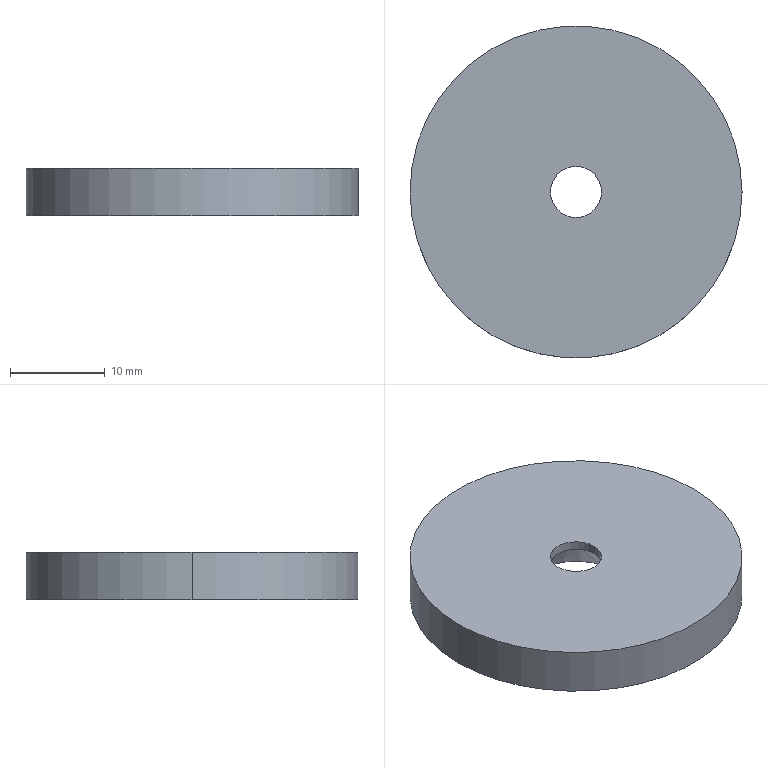Part | Creo | 1 solid | 8 faces | box 35 x 35 x 5 mm | volume 4524 mm3 | cylinder 4 | plane 2 | cone 2 | commonest cylinder face diameters 5.4 x2 35 x2
STEP:
#1=CARTESIAN_POINT('',(0.,0.,0.));
#2=DIRECTION('',(0.,0.,1.));
#3=DIRECTION('',(1.,0.,0.));
#4=AXIS2_PLACEMENT_3D('',#1,#2,#3);
#5=CARTESIAN_POINT('',(426.601,-277.627,-28.441));
#6=VERTEX_POINT('',#5);
#7=CARTESIAN_POINT('',(461.601,-277.627,-28.441));
#8=VERTEX_POINT('',#7);
#9=CARTESIAN_POINT('',(444.101,-277.627,-28.441));
#10=DIRECTION('',(0.,0.,-1.));
#11=DIRECTION('',(-1.,0.,0.));
#12=AXIS2_PLACEMENT_3D('',#9,#10,#11);
#13=CIRCLE('',#12,17.5);
#14=EDGE_CURVE('',#6,#8,#13,.T.);
#15=ORIENTED_EDGE('',*,*,#14,.F.);
#16=CARTESIAN_POINT('',(444.101,-277.627,-28.441));
#17=DIRECTION('',(0.,0.,-1.));
#18=DIRECTION('',(1.,0.,0.));
#19=AXIS2_PLACEMENT_3D('',#16,#17,#18);
#20=CIRCLE('',#19,17.5);
#21=EDGE_CURVE('',#8,#6,#20,.T.);
#22=ORIENTED_EDGE('',*,*,#21,.F.);
#23=EDGE_LOOP('',(#15,#22));
#24=FACE_OUTER_BOUND('',#23,.F.);
#25=CARTESIAN_POINT('',(450.309,-277.627,-28.441));
#26=VERTEX_POINT('',#25);
#27=CARTESIAN_POINT('',(437.892,-277.627,-28.441));
#28=VERTEX_POINT('',#27);
#29=CARTESIAN_POINT('',(444.101,-277.627,-28.441));
#30=DIRECTION('',(0.,0.,1.));
#31=DIRECTION('',(1.,0.,0.));
#32=AXIS2_PLACEMENT_3D('',#29,#30,#31);
#33=CIRCLE('',#32,6.209);
#34=EDGE_CURVE('',#26,#28,#33,.T.);
#35=ORIENTED_EDGE('',*,*,#34,.F.);
#36=CARTESIAN_POINT('',(444.101,-277.627,-28.441));
#37=DIRECTION('',(0.,0.,1.));
#38=DIRECTION('',(-1.,0.,0.));
#39=AXIS2_PLACEMENT_3D('',#36,#37,#38);
#40=CIRCLE('',#39,6.209);
#41=EDGE_CURVE('',#28,#26,#40,.T.);
#42=ORIENTED_EDGE('',*,*,#41,.F.);
#43=EDGE_LOOP('',(#35,#42));
#44=FACE_BOUND('',#43,.F.);
#45=CARTESIAN_POINT('',(444.101,-277.627,-28.441));
#46=DIRECTION('',(0.,0.,-1.));
#47=DIRECTION('',(-1.,0.,0.));
#48=AXIS2_PLACEMENT_3D('',#45,#46,#47);
#49=PLANE('',#48);
#50=ADVANCED_FACE('',(#24,#44),#49,.T.);
#51=CARTESIAN_POINT('',(446.801,-277.627,-24.405));
#52=VERTEX_POINT('',#51);
#53=CARTESIAN_POINT('',(441.401,-277.627,-24.405));
#54=VERTEX_POINT('',#53);
#55=CARTESIAN_POINT('',(444.101,-277.627,-24.405));
#56=DIRECTION('',(0.,0.,1.));
#57=DIRECTION('',(1.,0.,0.));
#58=AXIS2_PLACEMENT_3D('',#55,#56,#57);
#59=CIRCLE('',#58,2.7);
#60=EDGE_CURVE('',#52,#54,#59,.T.);
#61=ORIENTED_EDGE('',*,*,#60,.F.);
#62=CARTESIAN_POINT('',(446.801,-277.627,-24.405));
#63=DIRECTION('',(0.6561,0.,-0.7547));
#64=VECTOR('',#63,5.348);
#65=LINE('',#62,#64);
#66=EDGE_CURVE('',#52,#26,#65,.T.);
#67=ORIENTED_EDGE('',*,*,#66,.T.);
#68=ORIENTED_EDGE('',*,*,#34,.T.);
#69=CARTESIAN_POINT('',(441.401,-277.627,-24.405));
#70=DIRECTION('',(-0.6561,0.,-0.7547));
#71=VECTOR('',#70,5.348);
#72=LINE('',#69,#71);
#73=EDGE_CURVE('',#54,#28,#72,.T.);
#74=ORIENTED_EDGE('',*,*,#73,.F.);
#75=EDGE_LOOP('',(#61,#67,#68,#74));
#76=FACE_OUTER_BOUND('',#75,.F.);
#77=CARTESIAN_POINT('',(444.101,-277.627,-26.423));
#78=DIRECTION('',(0.,0.,-1.));
#79=DIRECTION('',(-1.,0.,0.));
#80=AXIS2_PLACEMENT_3D('',#77,#78,#79);
#81=CONICAL_SURFACE('',#80,4.454,41.);
#82=ADVANCED_FACE('',(#76),#81,.F.);
#83=CARTESIAN_POINT('',(441.401,-277.627,-23.441));
#84=VERTEX_POINT('',#83);
#85=CARTESIAN_POINT('',(446.801,-277.627,-23.441));
#86=VERTEX_POINT('',#85);
#87=CARTESIAN_POINT('',(444.101,-277.627,-23.441));
#88=DIRECTION('',(0.,0.,-1.));
#89=DIRECTION('',(-1.,0.,0.));
#90=AXIS2_PLACEMENT_3D('',#87,#88,#89);
#91=CIRCLE('',#90,2.7);
#92=EDGE_CURVE('',#84,#86,#91,.T.);
#93=ORIENTED_EDGE('',*,*,#92,.T.);
#94=CARTESIAN_POINT('',(446.801,-277.627,-23.441));
#95=DIRECTION('',(0.,0.,-1.));
#96=VECTOR('',#95,0.9639);
#97=LINE('',#94,#96);
#98=EDGE_CURVE('',#86,#52,#97,.T.);
#99=ORIENTED_EDGE('',*,*,#98,.T.);
#100=ORIENTED_EDGE('',*,*,#60,.T.);
#101=CARTESIAN_POINT('',(441.401,-277.627,-23.441));
#102=DIRECTION('',(0.,0.,-1.));
#103=VECTOR('',#102,0.9639);
#104=LINE('',#101,#103);
#105=EDGE_CURVE('',#84,#54,#104,.T.);
#106=ORIENTED_EDGE('',*,*,#105,.F.);
#107=EDGE_LOOP('',(#93,#99,#100,#106));
#108=FACE_OUTER_BOUND('',#107,.F.);
#109=CARTESIAN_POINT('',(444.101,-277.627,-23.441));
#110=DIRECTION('',(0.,0.,-1.));
#111=DIRECTION('',(-1.,0.,0.));
#112=AXIS2_PLACEMENT_3D('',#109,#110,#111);
#113=CYLINDRICAL_SURFACE('',#112,2.7);
#114=ADVANCED_FACE('',(#108),#113,.F.);
#115=CARTESIAN_POINT('',(461.601,-277.627,-23.441));
#116=VERTEX_POINT('',#115);
#117=CARTESIAN_POINT('',(426.601,-277.627,-23.441));
#118=VERTEX_POINT('',#117);
#119=CARTESIAN_POINT('',(444.101,-277.627,-23.441));
#120=DIRECTION('',(0.,0.,1.));
#121=DIRECTION('',(1.,0.,0.));
#122=AXIS2_PLACEMENT_3D('',#119,#120,#121);
#123=CIRCLE('',#122,17.5);
#124=EDGE_CURVE('',#116,#118,#123,.T.);
#125=ORIENTED_EDGE('',*,*,#124,.F.);
#126=CARTESIAN_POINT('',(444.101,-277.627,-23.441));
#127=DIRECTION('',(0.,0.,1.));
#128=DIRECTION('',(-1.,0.,0.));
#129=AXIS2_PLACEMENT_3D('',#126,#127,#128);
#130=CIRCLE('',#129,17.5);
#131=EDGE_CURVE('',#118,#116,#130,.T.);
#132=ORIENTED_EDGE('',*,*,#131,.F.);
#133=EDGE_LOOP('',(#125,#132));
#134=FACE_OUTER_BOUND('',#133,.F.);
#135=ORIENTED_EDGE('',*,*,#92,.F.);
#136=CARTESIAN_POINT('',(444.101,-277.627,-23.441));
#137=DIRECTION('',(0.,0.,-1.));
#138=DIRECTION('',(1.,0.,0.));
#139=AXIS2_PLACEMENT_3D('',#136,#137,#138);
#140=CIRCLE('',#139,2.7);
#141=EDGE_CURVE('',#86,#84,#140,.T.);
#142=ORIENTED_EDGE('',*,*,#141,.F.);
#143=EDGE_LOOP('',(#135,#142));
#144=FACE_BOUND('',#143,.F.);
#145=CARTESIAN_POINT('',(444.101,-277.627,-23.441));
#146=DIRECTION('',(0.,0.,1.));
#147=DIRECTION('',(1.,0.,0.));
#148=AXIS2_PLACEMENT_3D('',#145,#146,#147);
#149=PLANE('',#148);
#150=ADVANCED_FACE('',(#134,#144),#149,.T.);
#151=ORIENTED_EDGE('',*,*,#141,.T.);
#152=ORIENTED_EDGE('',*,*,#105,.T.);
#153=CARTESIAN_POINT('',(444.101,-277.627,-24.405));
#154=DIRECTION('',(0.,0.,1.));
#155=DIRECTION('',(-1.,0.,0.));
#156=AXIS2_PLACEMENT_3D('',#153,#154,#155);
#157=CIRCLE('',#156,2.7);
#158=EDGE_CURVE('',#54,#52,#157,.T.);
#159=ORIENTED_EDGE('',*,*,#158,.T.);
#160=ORIENTED_EDGE('',*,*,#98,.F.);
#161=EDGE_LOOP('',(#151,#152,#159,#160));
#162=FACE_OUTER_BOUND('',#161,.F.);
#163=CARTESIAN_POINT('',(444.101,-277.627,-23.441));
#164=DIRECTION('',(0.,0.,-1.));
#165=DIRECTION('',(-1.,0.,0.));
#166=AXIS2_PLACEMENT_3D('',#163,#164,#165);
#167=CYLINDRICAL_SURFACE('',#166,2.7);
#168=ADVANCED_FACE('',(#162),#167,.F.);
#169=ORIENTED_EDGE('',*,*,#158,.F.);
#170=ORIENTED_EDGE('',*,*,#73,.T.);
#171=ORIENTED_EDGE('',*,*,#41,.T.);
#172=ORIENTED_EDGE('',*,*,#66,.F.);
#173=EDGE_LOOP('',(#169,#170,#171,#172));
#174=FACE_OUTER_BOUND('',#173,.F.);
#175=CARTESIAN_POINT('',(444.101,-277.627,-26.423));
#176=DIRECTION('',(0.,0.,-1.));
#177=DIRECTION('',(-1.,0.,0.));
#178=AXIS2_PLACEMENT_3D('',#175,#176,#177);
#179=CONICAL_SURFACE('',#178,4.454,41.);
#180=ADVANCED_FACE('',(#174),#179,.F.);
#181=ORIENTED_EDGE('',*,*,#14,.T.);
#182=CARTESIAN_POINT('',(461.601,-277.627,-23.441));
#183=DIRECTION('',(0.,0.,-1.));
#184=VECTOR('',#183,5.);
#185=LINE('',#182,#184);
#186=EDGE_CURVE('',#116,#8,#185,.T.);
#187=ORIENTED_EDGE('',*,*,#186,.F.);
#188=ORIENTED_EDGE('',*,*,#124,.T.);
#189=CARTESIAN_POINT('',(426.601,-277.627,-23.441));
#190=DIRECTION('',(0.,0.,-1.));
#191=VECTOR('',#190,5.);
#192=LINE('',#189,#191);
#193=EDGE_CURVE('',#118,#6,#192,.T.);
#194=ORIENTED_EDGE('',*,*,#193,.T.);
#195=EDGE_LOOP('',(#181,#187,#188,#194));
#196=FACE_OUTER_BOUND('',#195,.F.);
#197=CARTESIAN_POINT('',(444.101,-277.627,-23.441));
#198=DIRECTION('',(0.,0.,-1.));
#199=DIRECTION('',(-1.,0.,0.));
#200=AXIS2_PLACEMENT_3D('',#197,#198,#199);
#201=CYLINDRICAL_SURFACE('',#200,17.5);
#202=ADVANCED_FACE('',(#196),#201,.T.);
#203=ORIENTED_EDGE('',*,*,#21,.T.);
#204=ORIENTED_EDGE('',*,*,#193,.F.);
#205=ORIENTED_EDGE('',*,*,#131,.T.);
#206=ORIENTED_EDGE('',*,*,#186,.T.);
#207=EDGE_LOOP('',(#203,#204,#205,#206));
#208=FACE_OUTER_BOUND('',#207,.F.);
#209=CARTESIAN_POINT('',(444.101,-277.627,-23.441));
#210=DIRECTION('',(0.,0.,-1.));
#211=DIRECTION('',(-1.,0.,0.));
#212=AXIS2_PLACEMENT_3D('',#209,#210,#211);
#213=CYLINDRICAL_SURFACE('',#212,17.5);
#214=ADVANCED_FACE('',(#208),#213,.T.);
#215=CLOSED_SHELL('',(#50,#82,#114,#150,#168,#180,#202,#214));
#216=MANIFOLD_SOLID_BREP('',#215);
#217=(LENGTH_UNIT()NAMED_UNIT(*)SI_UNIT(.MILLI.,.METRE.));
#218=UNCERTAINTY_MEASURE_WITH_UNIT(LENGTH_MEASURE(0.004976),#217,'','');
#219=(NAMED_UNIT(*)PLANE_ANGLE_UNIT()SI_UNIT($,.RADIAN.));
#220=PLANE_ANGLE_MEASURE_WITH_UNIT(PLANE_ANGLE_MEASURE(0.01745),#219);
#221=(CONVERSION_BASED_UNIT('DEGREE',#220)NAMED_UNIT(*)PLANE_ANGLE_UNIT());
#222=(NAMED_UNIT(*)SI_UNIT($,.STERADIAN.)SOLID_ANGLE_UNIT());
#223=(GEOMETRIC_REPRESENTATION_CONTEXT(3)GLOBAL_UNCERTAINTY_ASSIGNED_CONTEXT((#218))GLOBAL_UNIT_ASSIGNED_CONTEXT((#217,#221,#222))REPRESENTATION_CONTEXT('',''));
#224=ADVANCED_BREP_SHAPE_REPRESENTATION('',(#4,#216),#223);